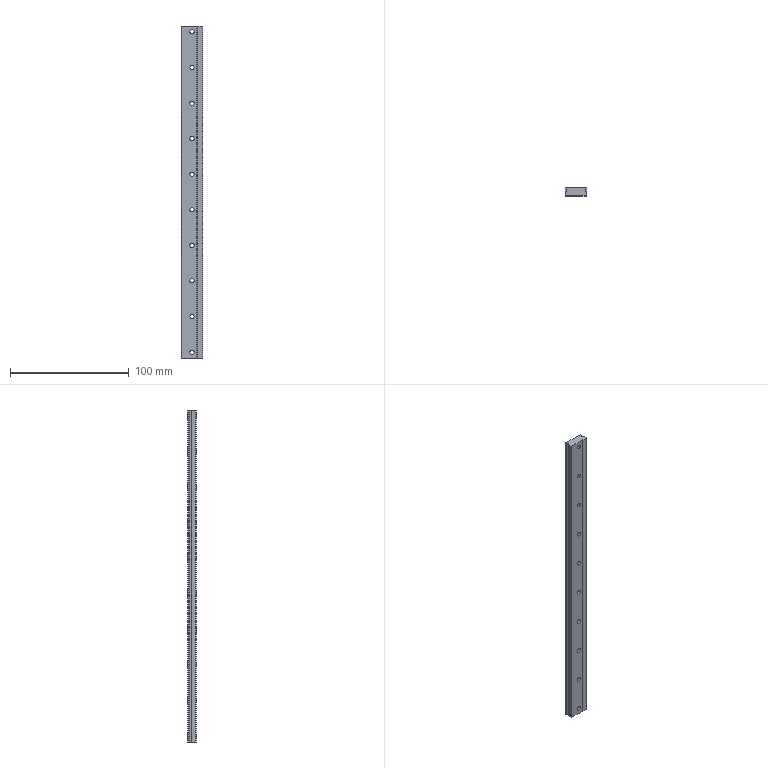Part | NX | features BREP 1 | 1 solid | 67 faces | box 18 x 7 x 280 mm | volume 32694 mm3 | cylinder 44 | plane 23 | commonest cylinder face diameters 3.5 x20 6.5 x20 2 x3 0.6 x1